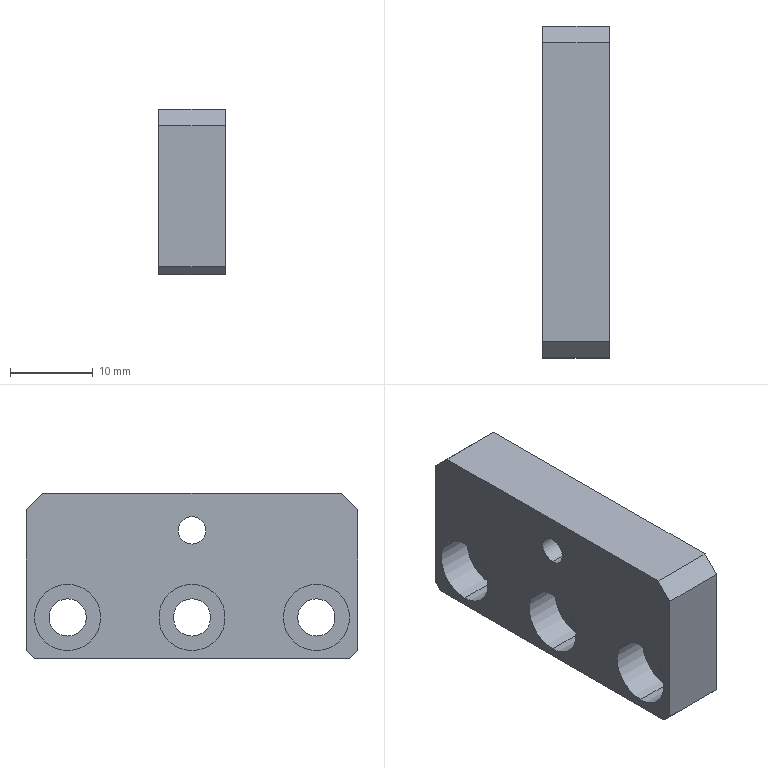Part | STEP file | 11-FG-E04511 | 1 solid | 27 faces | box 8 x 40 x 20 mm | volume 5456 mm3 | cylinder 14 | plane 13 | commonest cylinder face diameters 4.5 x6 8 x6 3.3 x2
STEP:
#1=CARTESIAN_POINT('',(4.,0.,13.85));
#2=VERTEX_POINT('',#1);
#3=CARTESIAN_POINT('',(4.,0.,17.15));
#4=VERTEX_POINT('',#3);
#5=CARTESIAN_POINT('',(4.,0.,15.5));
#6=DIRECTION('',(-1.,0.,0.));
#7=DIRECTION('',(0.,-1.,0.));
#8=AXIS2_PLACEMENT_3D('',#5,#6,#7);
#9=CIRCLE('',#8,1.65);
#10=EDGE_CURVE('',#2,#4,#9,.T.);
#11=ORIENTED_EDGE('',*,*,#10,.F.);
#12=CARTESIAN_POINT('',(-4.,0.,13.85));
#13=VERTEX_POINT('',#12);
#14=CARTESIAN_POINT('',(-4.,0.,13.85));
#15=DIRECTION('',(-1.,0.,0.));
#16=VECTOR('',#15,1000.);
#17=LINE('',#14,#16);
#18=EDGE_CURVE('',#2,#13,#17,.T.);
#19=ORIENTED_EDGE('',*,*,#18,.T.);
#20=CARTESIAN_POINT('',(-4.,0.,17.15));
#21=VERTEX_POINT('',#20);
#22=CARTESIAN_POINT('',(-4.,0.,15.5));
#23=DIRECTION('',(-1.,0.,0.));
#24=DIRECTION('',(0.,0.,1.));
#25=AXIS2_PLACEMENT_3D('',#22,#23,#24);
#26=CIRCLE('',#25,1.65);
#27=EDGE_CURVE('',#13,#21,#26,.T.);
#28=ORIENTED_EDGE('',*,*,#27,.T.);
#29=CARTESIAN_POINT('',(-4.,0.,17.15));
#30=DIRECTION('',(-1.,0.,0.));
#31=VECTOR('',#30,1000.);
#32=LINE('',#29,#31);
#33=EDGE_CURVE('',#4,#21,#32,.T.);
#34=ORIENTED_EDGE('',*,*,#33,.F.);
#35=EDGE_LOOP('',(#11,#19,#28,#34));
#36=FACE_OUTER_BOUND('',#35,.T.);
#37=CARTESIAN_POINT('',(-4.,0.,15.5));
#38=DIRECTION('',(-1.,0.,0.));
#39=DIRECTION('',(0.,0.,1.));
#40=AXIS2_PLACEMENT_3D('',#37,#38,#39);
#41=CYLINDRICAL_SURFACE('',#40,1.65);
#42=ADVANCED_FACE('',(#36),#41,.F.);
#43=CARTESIAN_POINT('',(0.4,15.,1.));
#44=VERTEX_POINT('',#43);
#45=CARTESIAN_POINT('',(0.4,15.,9.));
#46=VERTEX_POINT('',#45);
#47=CARTESIAN_POINT('',(0.4,15.,5.));
#48=DIRECTION('',(-1.,0.,0.));
#49=DIRECTION('',(0.,0.,1.));
#50=AXIS2_PLACEMENT_3D('',#47,#48,#49);
#51=CIRCLE('',#50,4.);
#52=EDGE_CURVE('',#44,#46,#51,.T.);
#53=ORIENTED_EDGE('',*,*,#52,.F.);
#54=CARTESIAN_POINT('',(-4.,15.,1.));
#55=VERTEX_POINT('',#54);
#56=CARTESIAN_POINT('',(-4.,15.,1.));
#57=DIRECTION('',(-1.,0.,0.));
#58=VECTOR('',#57,1000.);
#59=LINE('',#56,#58);
#60=EDGE_CURVE('',#44,#55,#59,.T.);
#61=ORIENTED_EDGE('',*,*,#60,.T.);
#62=CARTESIAN_POINT('',(-4.,15.,9.));
#63=VERTEX_POINT('',#62);
#64=CARTESIAN_POINT('',(-4.,15.,5.));
#65=DIRECTION('',(-1.,0.,0.));
#66=DIRECTION('',(0.,0.,1.));
#67=AXIS2_PLACEMENT_3D('',#64,#65,#66);
#68=CIRCLE('',#67,4.);
#69=EDGE_CURVE('',#55,#63,#68,.T.);
#70=ORIENTED_EDGE('',*,*,#69,.T.);
#71=CARTESIAN_POINT('',(-4.,15.,9.));
#72=DIRECTION('',(-1.,0.,0.));
#73=VECTOR('',#72,1000.);
#74=LINE('',#71,#73);
#75=EDGE_CURVE('',#46,#63,#74,.T.);
#76=ORIENTED_EDGE('',*,*,#75,.F.);
#77=EDGE_LOOP('',(#53,#61,#70,#76));
#78=FACE_OUTER_BOUND('',#77,.T.);
#79=CARTESIAN_POINT('',(-4.,15.,5.));
#80=DIRECTION('',(-1.,0.,0.));
#81=DIRECTION('',(0.,0.,1.));
#82=AXIS2_PLACEMENT_3D('',#79,#80,#81);
#83=CYLINDRICAL_SURFACE('',#82,4.);
#84=ADVANCED_FACE('',(#78),#83,.F.);
#85=CARTESIAN_POINT('',(4.,15.,2.75));
#86=VERTEX_POINT('',#85);
#87=CARTESIAN_POINT('',(4.,15.,7.25));
#88=VERTEX_POINT('',#87);
#89=CARTESIAN_POINT('',(4.,15.,5.));
#90=DIRECTION('',(-1.,0.,0.));
#91=DIRECTION('',(0.,-1.,0.));
#92=AXIS2_PLACEMENT_3D('',#89,#90,#91);
#93=CIRCLE('',#92,2.25);
#94=EDGE_CURVE('',#86,#88,#93,.T.);
#95=ORIENTED_EDGE('',*,*,#94,.F.);
#96=CARTESIAN_POINT('',(0.4,15.,2.75));
#97=VERTEX_POINT('',#96);
#98=CARTESIAN_POINT('',(-4.,15.,2.75));
#99=DIRECTION('',(-1.,0.,0.));
#100=VECTOR('',#99,1000.);
#101=LINE('',#98,#100);
#102=EDGE_CURVE('',#86,#97,#101,.T.);
#103=ORIENTED_EDGE('',*,*,#102,.T.);
#104=CARTESIAN_POINT('',(0.4,15.,7.25));
#105=VERTEX_POINT('',#104);
#106=CARTESIAN_POINT('',(0.4,15.,5.));
#107=DIRECTION('',(-1.,0.,0.));
#108=DIRECTION('',(0.,0.,1.));
#109=AXIS2_PLACEMENT_3D('',#106,#107,#108);
#110=CIRCLE('',#109,2.25);
#111=EDGE_CURVE('',#97,#105,#110,.T.);
#112=ORIENTED_EDGE('',*,*,#111,.T.);
#113=CARTESIAN_POINT('',(-4.,15.,7.25));
#114=DIRECTION('',(-1.,0.,0.));
#115=VECTOR('',#114,1000.);
#116=LINE('',#113,#115);
#117=EDGE_CURVE('',#88,#105,#116,.T.);
#118=ORIENTED_EDGE('',*,*,#117,.F.);
#119=EDGE_LOOP('',(#95,#103,#112,#118));
#120=FACE_OUTER_BOUND('',#119,.T.);
#121=CARTESIAN_POINT('',(-4.,15.,5.));
#122=DIRECTION('',(-1.,0.,0.));
#123=DIRECTION('',(0.,0.,1.));
#124=AXIS2_PLACEMENT_3D('',#121,#122,#123);
#125=CYLINDRICAL_SURFACE('',#124,2.25);
#126=ADVANCED_FACE('',(#120),#125,.F.);
#127=CARTESIAN_POINT('',(0.4,0.,1.));
#128=VERTEX_POINT('',#127);
#129=CARTESIAN_POINT('',(0.4,0.,9.));
#130=VERTEX_POINT('',#129);
#131=CARTESIAN_POINT('',(0.4,0.,5.));
#132=DIRECTION('',(-1.,0.,0.));
#133=DIRECTION('',(0.,0.,1.));
#134=AXIS2_PLACEMENT_3D('',#131,#132,#133);
#135=CIRCLE('',#134,4.);
#136=EDGE_CURVE('',#128,#130,#135,.T.);
#137=ORIENTED_EDGE('',*,*,#136,.F.);
#138=CARTESIAN_POINT('',(-4.,0.,1.));
#139=VERTEX_POINT('',#138);
#140=CARTESIAN_POINT('',(-4.,0.,1.));
#141=DIRECTION('',(-1.,0.,0.));
#142=VECTOR('',#141,1000.);
#143=LINE('',#140,#142);
#144=EDGE_CURVE('',#128,#139,#143,.T.);
#145=ORIENTED_EDGE('',*,*,#144,.T.);
#146=CARTESIAN_POINT('',(-4.,0.,9.));
#147=VERTEX_POINT('',#146);
#148=CARTESIAN_POINT('',(-4.,0.,5.));
#149=DIRECTION('',(-1.,0.,0.));
#150=DIRECTION('',(0.,0.,1.));
#151=AXIS2_PLACEMENT_3D('',#148,#149,#150);
#152=CIRCLE('',#151,4.);
#153=EDGE_CURVE('',#139,#147,#152,.T.);
#154=ORIENTED_EDGE('',*,*,#153,.T.);
#155=CARTESIAN_POINT('',(-4.,0.,9.));
#156=DIRECTION('',(-1.,0.,0.));
#157=VECTOR('',#156,1000.);
#158=LINE('',#155,#157);
#159=EDGE_CURVE('',#130,#147,#158,.T.);
#160=ORIENTED_EDGE('',*,*,#159,.F.);
#161=EDGE_LOOP('',(#137,#145,#154,#160));
#162=FACE_OUTER_BOUND('',#161,.T.);
#163=CARTESIAN_POINT('',(-4.,0.,5.));
#164=DIRECTION('',(-1.,0.,0.));
#165=DIRECTION('',(0.,0.,1.));
#166=AXIS2_PLACEMENT_3D('',#163,#164,#165);
#167=CYLINDRICAL_SURFACE('',#166,4.);
#168=ADVANCED_FACE('',(#162),#167,.F.);
#169=CARTESIAN_POINT('',(4.,0.,2.75));
#170=VERTEX_POINT('',#169);
#171=CARTESIAN_POINT('',(4.,0.,7.25));
#172=VERTEX_POINT('',#171);
#173=CARTESIAN_POINT('',(4.,0.,5.));
#174=DIRECTION('',(-1.,0.,0.));
#175=DIRECTION('',(0.,-1.,0.));
#176=AXIS2_PLACEMENT_3D('',#173,#174,#175);
#177=CIRCLE('',#176,2.25);
#178=EDGE_CURVE('',#170,#172,#177,.T.);
#179=ORIENTED_EDGE('',*,*,#178,.F.);
#180=CARTESIAN_POINT('',(0.4,0.,2.75));
#181=VERTEX_POINT('',#180);
#182=CARTESIAN_POINT('',(-4.,0.,2.75));
#183=DIRECTION('',(-1.,0.,0.));
#184=VECTOR('',#183,1000.);
#185=LINE('',#182,#184);
#186=EDGE_CURVE('',#170,#181,#185,.T.);
#187=ORIENTED_EDGE('',*,*,#186,.T.);
#188=CARTESIAN_POINT('',(0.4,0.,7.25));
#189=VERTEX_POINT('',#188);
#190=CARTESIAN_POINT('',(0.4,0.,5.));
#191=DIRECTION('',(-1.,0.,0.));
#192=DIRECTION('',(0.,0.,1.));
#193=AXIS2_PLACEMENT_3D('',#190,#191,#192);
#194=CIRCLE('',#193,2.25);
#195=EDGE_CURVE('',#181,#189,#194,.T.);
#196=ORIENTED_EDGE('',*,*,#195,.T.);
#197=CARTESIAN_POINT('',(-4.,0.,7.25));
#198=DIRECTION('',(-1.,0.,0.));
#199=VECTOR('',#198,1000.);
#200=LINE('',#197,#199);
#201=EDGE_CURVE('',#172,#189,#200,.T.);
#202=ORIENTED_EDGE('',*,*,#201,.F.);
#203=EDGE_LOOP('',(#179,#187,#196,#202));
#204=FACE_OUTER_BOUND('',#203,.T.);
#205=CARTESIAN_POINT('',(-4.,0.,5.));
#206=DIRECTION('',(-1.,0.,0.));
#207=DIRECTION('',(0.,0.,1.));
#208=AXIS2_PLACEMENT_3D('',#205,#206,#207);
#209=CYLINDRICAL_SURFACE('',#208,2.25);
#210=ADVANCED_FACE('',(#204),#209,.F.);
#211=CARTESIAN_POINT('',(0.4,-15.,1.));
#212=VERTEX_POINT('',#211);
#213=CARTESIAN_POINT('',(0.4,-15.,9.));
#214=VERTEX_POINT('',#213);
#215=CARTESIAN_POINT('',(0.4,-15.,5.));
#216=DIRECTION('',(-1.,0.,0.));
#217=DIRECTION('',(0.,0.,1.));
#218=AXIS2_PLACEMENT_3D('',#215,#216,#217);
#219=CIRCLE('',#218,4.);
#220=EDGE_CURVE('',#212,#214,#219,.T.);
#221=ORIENTED_EDGE('',*,*,#220,.F.);
#222=CARTESIAN_POINT('',(-4.,-15.,1.));
#223=VERTEX_POINT('',#222);
#224=CARTESIAN_POINT('',(-4.,-15.,1.));
#225=DIRECTION('',(-1.,0.,0.));
#226=VECTOR('',#225,1000.);
#227=LINE('',#224,#226);
#228=EDGE_CURVE('',#212,#223,#227,.T.);
#229=ORIENTED_EDGE('',*,*,#228,.T.);
#230=CARTESIAN_POINT('',(-4.,-15.,9.));
#231=VERTEX_POINT('',#230);
#232=CARTESIAN_POINT('',(-4.,-15.,5.));
#233=DIRECTION('',(-1.,0.,0.));
#234=DIRECTION('',(0.,0.,1.));
#235=AXIS2_PLACEMENT_3D('',#232,#233,#234);
#236=CIRCLE('',#235,4.);
#237=EDGE_CURVE('',#223,#231,#236,.T.);
#238=ORIENTED_EDGE('',*,*,#237,.T.);
#239=CARTESIAN_POINT('',(-4.,-15.,9.));
#240=DIRECTION('',(-1.,0.,0.));
#241=VECTOR('',#240,1000.);
#242=LINE('',#239,#241);
#243=EDGE_CURVE('',#214,#231,#242,.T.);
#244=ORIENTED_EDGE('',*,*,#243,.F.);
#245=EDGE_LOOP('',(#221,#229,#238,#244));
#246=FACE_OUTER_BOUND('',#245,.T.);
#247=CARTESIAN_POINT('',(-4.,-15.,5.));
#248=DIRECTION('',(-1.,0.,0.));
#249=DIRECTION('',(0.,0.,1.));
#250=AXIS2_PLACEMENT_3D('',#247,#248,#249);
#251=CYLINDRICAL_SURFACE('',#250,4.);
#252=ADVANCED_FACE('',(#246),#251,.F.);
#253=CARTESIAN_POINT('',(4.,-15.,2.75));
#254=VERTEX_POINT('',#253);
#255=CARTESIAN_POINT('',(4.,-15.,7.25));
#256=VERTEX_POINT('',#255);
#257=CARTESIAN_POINT('',(4.,-15.,5.));
#258=DIRECTION('',(-1.,0.,0.));
#259=DIRECTION('',(0.,-1.,0.));
#260=AXIS2_PLACEMENT_3D('',#257,#258,#259);
#261=CIRCLE('',#260,2.25);
#262=EDGE_CURVE('',#254,#256,#261,.T.);
#263=ORIENTED_EDGE('',*,*,#262,.F.);
#264=CARTESIAN_POINT('',(0.4,-15.,2.75));
#265=VERTEX_POINT('',#264);
#266=CARTESIAN_POINT('',(-4.,-15.,2.75));
#267=DIRECTION('',(-1.,0.,0.));
#268=VECTOR('',#267,1000.);
#269=LINE('',#266,#268);
#270=EDGE_CURVE('',#254,#265,#269,.T.);
#271=ORIENTED_EDGE('',*,*,#270,.T.);
#272=CARTESIAN_POINT('',(0.4,-15.,7.25));
#273=VERTEX_POINT('',#272);
#274=CARTESIAN_POINT('',(0.4,-15.,5.));
#275=DIRECTION('',(-1.,0.,0.));
#276=DIRECTION('',(0.,0.,1.));
#277=AXIS2_PLACEMENT_3D('',#274,#275,#276);
#278=CIRCLE('',#277,2.25);
#279=EDGE_CURVE('',#265,#273,#278,.T.);
#280=ORIENTED_EDGE('',*,*,#279,.T.);
#281=CARTESIAN_POINT('',(-4.,-15.,7.25));
#282=DIRECTION('',(-1.,0.,0.));
#283=VECTOR('',#282,1000.);
#284=LINE('',#281,#283);
#285=EDGE_CURVE('',#256,#273,#284,.T.);
#286=ORIENTED_EDGE('',*,*,#285,.F.);
#287=EDGE_LOOP('',(#263,#271,#280,#286));
#288=FACE_OUTER_BOUND('',#287,.T.);
#289=CARTESIAN_POINT('',(-4.,-15.,5.));
#290=DIRECTION('',(-1.,0.,0.));
#291=DIRECTION('',(0.,0.,1.));
#292=AXIS2_PLACEMENT_3D('',#289,#290,#291);
#293=CYLINDRICAL_SURFACE('',#292,2.25);
#294=ADVANCED_FACE('',(#288),#293,.F.);
#295=CARTESIAN_POINT('',(4.,0.,15.5));
#296=DIRECTION('',(-1.,0.,0.));
#297=DIRECTION('',(0.,-1.,0.));
#298=AXIS2_PLACEMENT_3D('',#295,#296,#297);
#299=CIRCLE('',#298,1.65);
#300=EDGE_CURVE('',#4,#2,#299,.T.);
#301=ORIENTED_EDGE('',*,*,#300,.T.);
#302=ORIENTED_EDGE('',*,*,#10,.T.);
#303=EDGE_LOOP('',(#301,#302));
#304=FACE_BOUND('',#303,.T.);
#305=CARTESIAN_POINT('',(4.,15.,5.));
#306=DIRECTION('',(-1.,0.,0.));
#307=DIRECTION('',(0.,-1.,0.));
#308=AXIS2_PLACEMENT_3D('',#305,#306,#307);
#309=CIRCLE('',#308,2.25);
#310=EDGE_CURVE('',#88,#86,#309,.T.);
#311=ORIENTED_EDGE('',*,*,#310,.T.);
#312=ORIENTED_EDGE('',*,*,#94,.T.);
#313=EDGE_LOOP('',(#311,#312));
#314=FACE_BOUND('',#313,.T.);
#315=CARTESIAN_POINT('',(4.,0.,5.));
#316=DIRECTION('',(-1.,0.,0.));
#317=DIRECTION('',(0.,-1.,0.));
#318=AXIS2_PLACEMENT_3D('',#315,#316,#317);
#319=CIRCLE('',#318,2.25);
#320=EDGE_CURVE('',#172,#170,#319,.T.);
#321=ORIENTED_EDGE('',*,*,#320,.T.);
#322=ORIENTED_EDGE('',*,*,#178,.T.);
#323=EDGE_LOOP('',(#321,#322));
#324=FACE_BOUND('',#323,.T.);
#325=CARTESIAN_POINT('',(4.,-15.,5.));
#326=DIRECTION('',(-1.,0.,0.));
#327=DIRECTION('',(0.,-1.,0.));
#328=AXIS2_PLACEMENT_3D('',#325,#326,#327);
#329=CIRCLE('',#328,2.25);
#330=EDGE_CURVE('',#256,#254,#329,.T.);
#331=ORIENTED_EDGE('',*,*,#330,.T.);
#332=ORIENTED_EDGE('',*,*,#262,.T.);
#333=EDGE_LOOP('',(#331,#332));
#334=FACE_BOUND('',#333,.T.);
#335=CARTESIAN_POINT('',(4.,-20.,18.));
#336=VERTEX_POINT('',#335);
#337=CARTESIAN_POINT('',(4.,-20.,1.));
#338=VERTEX_POINT('',#337);
#339=CARTESIAN_POINT('',(4.,-20.,20.));
#340=DIRECTION('',(0.,0.,-1.));
#341=VECTOR('',#340,1000.);
#342=LINE('',#339,#341);
#343=EDGE_CURVE('',#336,#338,#342,.T.);
#344=ORIENTED_EDGE('',*,*,#343,.T.);
#345=CARTESIAN_POINT('',(4.,-19.,0.));
#346=VERTEX_POINT('',#345);
#347=CARTESIAN_POINT('',(4.,-20.,1.));
#348=DIRECTION('',(0.,0.7071,-0.7071));
#349=VECTOR('',#348,1000.);
#350=LINE('',#347,#349);
#351=EDGE_CURVE('',#338,#346,#350,.T.);
#352=ORIENTED_EDGE('',*,*,#351,.T.);
#353=CARTESIAN_POINT('',(4.,19.,0.));
#354=VERTEX_POINT('',#353);
#355=CARTESIAN_POINT('',(4.,20.,0.));
#356=DIRECTION('',(0.,1.,0.));
#357=VECTOR('',#356,1000.);
#358=LINE('',#355,#357);
#359=EDGE_CURVE('',#346,#354,#358,.T.);
#360=ORIENTED_EDGE('',*,*,#359,.T.);
#361=CARTESIAN_POINT('',(4.,20.,1.));
#362=VERTEX_POINT('',#361);
#363=CARTESIAN_POINT('',(4.,20.,1.));
#364=DIRECTION('',(0.,0.7071,0.7071));
#365=VECTOR('',#364,1000.);
#366=LINE('',#363,#365);
#367=EDGE_CURVE('',#354,#362,#366,.T.);
#368=ORIENTED_EDGE('',*,*,#367,.T.);
#369=CARTESIAN_POINT('',(4.,20.,18.));
#370=VERTEX_POINT('',#369);
#371=CARTESIAN_POINT('',(4.,20.,20.));
#372=DIRECTION('',(0.,0.,-1.));
#373=VECTOR('',#372,1000.);
#374=LINE('',#371,#373);
#375=EDGE_CURVE('',#370,#362,#374,.T.);
#376=ORIENTED_EDGE('',*,*,#375,.F.);
#377=CARTESIAN_POINT('',(4.,18.,20.));
#378=VERTEX_POINT('',#377);
#379=CARTESIAN_POINT('',(4.,18.,20.));
#380=DIRECTION('',(0.,-0.7071,0.7071));
#381=VECTOR('',#380,1000.);
#382=LINE('',#379,#381);
#383=EDGE_CURVE('',#370,#378,#382,.T.);
#384=ORIENTED_EDGE('',*,*,#383,.T.);
#385=CARTESIAN_POINT('',(4.,-18.,20.));
#386=VERTEX_POINT('',#385);
#387=CARTESIAN_POINT('',(4.,20.,20.));
#388=DIRECTION('',(0.,1.,0.));
#389=VECTOR('',#388,1000.);
#390=LINE('',#387,#389);
#391=EDGE_CURVE('',#386,#378,#390,.T.);
#392=ORIENTED_EDGE('',*,*,#391,.F.);
#393=CARTESIAN_POINT('',(4.,-18.,20.));
#394=DIRECTION('',(0.,-0.7071,-0.7071));
#395=VECTOR('',#394,1000.);
#396=LINE('',#393,#395);
#397=EDGE_CURVE('',#386,#336,#396,.T.);
#398=ORIENTED_EDGE('',*,*,#397,.T.);
#399=EDGE_LOOP('',(#344,#352,#360,#368,#376,#384,#392,#398));
#400=FACE_OUTER_BOUND('',#399,.T.);
#401=CARTESIAN_POINT('',(4.,20.,20.));
#402=DIRECTION('',(-1.,0.,0.));
#403=DIRECTION('',(0.,-1.,0.));
#404=AXIS2_PLACEMENT_3D('',#401,#402,#403);
#405=PLANE('',#404);
#406=ADVANCED_FACE('',(#304,#314,#324,#334,#400),#405,.F.);
#407=ORIENTED_EDGE('',*,*,#375,.T.);
#408=CARTESIAN_POINT('',(-4.,20.,1.));
#409=VERTEX_POINT('',#408);
#410=CARTESIAN_POINT('',(-4.,20.,1.));
#411=DIRECTION('',(-1.,0.,0.));
#412=VECTOR('',#411,1000.);
#413=LINE('',#410,#412);
#414=EDGE_CURVE('',#362,#409,#413,.T.);
#415=ORIENTED_EDGE('',*,*,#414,.T.);
#416=CARTESIAN_POINT('',(-4.,20.,18.));
#417=VERTEX_POINT('',#416);
#418=CARTESIAN_POINT('',(-4.,20.,20.));
#419=DIRECTION('',(0.,0.,-1.));
#420=VECTOR('',#419,1000.);
#421=LINE('',#418,#420);
#422=EDGE_CURVE('',#417,#409,#421,.T.);
#423=ORIENTED_EDGE('',*,*,#422,.F.);
#424=CARTESIAN_POINT('',(4.,20.,18.));
#425=DIRECTION('',(1.,0.,0.));
#426=VECTOR('',#425,1000.);
#427=LINE('',#424,#426);
#428=EDGE_CURVE('',#417,#370,#427,.T.);
#429=ORIENTED_EDGE('',*,*,#428,.T.);
#430=EDGE_LOOP('',(#407,#415,#423,#429));
#431=FACE_OUTER_BOUND('',#430,.T.);
#432=CARTESIAN_POINT('',(-4.,20.,20.));
#433=DIRECTION('',(0.,-1.,0.));
#434=DIRECTION('',(0.,0.,-1.));
#435=AXIS2_PLACEMENT_3D('',#432,#433,#434);
#436=PLANE('',#435);
#437=ADVANCED_FACE('',(#431),#436,.F.);
#438=CARTESIAN_POINT('',(-4.,0.,15.5));
#439=DIRECTION('',(-1.,0.,0.));
#440=DIRECTION('',(0.,0.,1.));
#441=AXIS2_PLACEMENT_3D('',#438,#439,#440);
#442=CIRCLE('',#441,1.65);
#443=EDGE_CURVE('',#21,#13,#442,.T.);
#444=ORIENTED_EDGE('',*,*,#443,.F.);
#445=ORIENTED_EDGE('',*,*,#27,.F.);
#446=EDGE_LOOP('',(#444,#445));
#447=FACE_BOUND('',#446,.T.);
#448=CARTESIAN_POINT('',(-4.,15.,5.));
#449=DIRECTION('',(-1.,0.,0.));
#450=DIRECTION('',(0.,0.,1.));
#451=AXIS2_PLACEMENT_3D('',#448,#449,#450);
#452=CIRCLE('',#451,4.);
#453=EDGE_CURVE('',#63,#55,#452,.T.);
#454=ORIENTED_EDGE('',*,*,#453,.F.);
#455=ORIENTED_EDGE('',*,*,#69,.F.);
#456=EDGE_LOOP('',(#454,#455));
#457=FACE_BOUND('',#456,.T.);
#458=CARTESIAN_POINT('',(-4.,0.,5.));
#459=DIRECTION('',(-1.,0.,0.));
#460=DIRECTION('',(0.,0.,1.));
#461=AXIS2_PLACEMENT_3D('',#458,#459,#460);
#462=CIRCLE('',#461,4.);
#463=EDGE_CURVE('',#147,#139,#462,.T.);
#464=ORIENTED_EDGE('',*,*,#463,.F.);
#465=ORIENTED_EDGE('',*,*,#153,.F.);
#466=EDGE_LOOP('',(#464,#465));
#467=FACE_BOUND('',#466,.T.);
#468=CARTESIAN_POINT('',(-4.,-15.,5.));
#469=DIRECTION('',(-1.,0.,0.));
#470=DIRECTION('',(0.,0.,1.));
#471=AXIS2_PLACEMENT_3D('',#468,#469,#470);
#472=CIRCLE('',#471,4.);
#473=EDGE_CURVE('',#231,#223,#472,.T.);
#474=ORIENTED_EDGE('',*,*,#473,.F.);
#475=ORIENTED_EDGE('',*,*,#237,.F.);
#476=EDGE_LOOP('',(#474,#475));
#477=FACE_BOUND('',#476,.T.);
#478=CARTESIAN_POINT('',(-4.,19.,0.));
#479=VERTEX_POINT('',#478);
#480=CARTESIAN_POINT('',(-4.,-19.,0.));
#481=VERTEX_POINT('',#480);
#482=CARTESIAN_POINT('',(-4.,20.,0.));
#483=DIRECTION('',(0.,-1.,0.));
#484=VECTOR('',#483,1000.);
#485=LINE('',#482,#484);
#486=EDGE_CURVE('',#479,#481,#485,.T.);
#487=ORIENTED_EDGE('',*,*,#486,.T.);
#488=CARTESIAN_POINT('',(-4.,-20.,1.));
#489=VERTEX_POINT('',#488);
#490=CARTESIAN_POINT('',(-4.,-20.,1.));
#491=DIRECTION('',(0.,-0.7071,0.7071));
#492=VECTOR('',#491,1000.);
#493=LINE('',#490,#492);
#494=EDGE_CURVE('',#481,#489,#493,.T.);
#495=ORIENTED_EDGE('',*,*,#494,.T.);
#496=CARTESIAN_POINT('',(-4.,-20.,18.));
#497=VERTEX_POINT('',#496);
#498=CARTESIAN_POINT('',(-4.,-20.,20.));
#499=DIRECTION('',(0.,0.,-1.));
#500=VECTOR('',#499,1000.);
#501=LINE('',#498,#500);
#502=EDGE_CURVE('',#497,#489,#501,.T.);
#503=ORIENTED_EDGE('',*,*,#502,.F.);
#504=CARTESIAN_POINT('',(-4.,-18.,20.));
#505=VERTEX_POINT('',#504);
#506=CARTESIAN_POINT('',(-4.,-18.,20.));
#507=DIRECTION('',(0.,0.7071,0.7071));
#508=VECTOR('',#507,1000.);
#509=LINE('',#506,#508);
#510=EDGE_CURVE('',#497,#505,#509,.T.);
#511=ORIENTED_EDGE('',*,*,#510,.T.);
#512=CARTESIAN_POINT('',(-4.,18.,20.));
#513=VERTEX_POINT('',#512);
#514=CARTESIAN_POINT('',(-4.,20.,20.));
#515=DIRECTION('',(0.,-1.,0.));
#516=VECTOR('',#515,1000.);
#517=LINE('',#514,#516);
#518=EDGE_CURVE('',#513,#505,#517,.T.);
#519=ORIENTED_EDGE('',*,*,#518,.F.);
#520=CARTESIAN_POINT('',(-4.,18.,20.));
#521=DIRECTION('',(0.,0.7071,-0.7071));
#522=VECTOR('',#521,1000.);
#523=LINE('',#520,#522);
#524=EDGE_CURVE('',#513,#417,#523,.T.);
#525=ORIENTED_EDGE('',*,*,#524,.T.);
#526=ORIENTED_EDGE('',*,*,#422,.T.);
#527=CARTESIAN_POINT('',(-4.,20.,1.));
#528=DIRECTION('',(0.,-0.7071,-0.7071));
#529=VECTOR('',#528,1000.);
#530=LINE('',#527,#529);
#531=EDGE_CURVE('',#409,#479,#530,.T.);
#532=ORIENTED_EDGE('',*,*,#531,.T.);
#533=EDGE_LOOP('',(#487,#495,#503,#511,#519,#525,#526,#532));
#534=FACE_OUTER_BOUND('',#533,.T.);
#535=CARTESIAN_POINT('',(-4.,20.,20.));
#536=DIRECTION('',(1.,0.,0.));
#537=DIRECTION('',(0.,1.,0.));
#538=AXIS2_PLACEMENT_3D('',#535,#536,#537);
#539=PLANE('',#538);
#540=ADVANCED_FACE('',(#447,#457,#467,#477,#534),#539,.F.);
#541=ORIENTED_EDGE('',*,*,#502,.T.);
#542=CARTESIAN_POINT('',(-4.,-20.,1.));
#543=DIRECTION('',(1.,0.,0.));
#544=VECTOR('',#543,1000.);
#545=LINE('',#542,#544);
#546=EDGE_CURVE('',#489,#338,#545,.T.);
#547=ORIENTED_EDGE('',*,*,#546,.T.);
#548=ORIENTED_EDGE('',*,*,#343,.F.);
#549=CARTESIAN_POINT('',(-4.,-20.,18.));
#550=DIRECTION('',(-1.,0.,0.));
#551=VECTOR('',#550,1000.);
#552=LINE('',#549,#551);
#553=EDGE_CURVE('',#336,#497,#552,.T.);
#554=ORIENTED_EDGE('',*,*,#553,.T.);
#555=EDGE_LOOP('',(#541,#547,#548,#554));
#556=FACE_OUTER_BOUND('',#555,.T.);
#557=CARTESIAN_POINT('',(-4.,-20.,20.));
#558=DIRECTION('',(0.,1.,0.));
#559=DIRECTION('',(0.,0.,1.));
#560=AXIS2_PLACEMENT_3D('',#557,#558,#559);
#561=PLANE('',#560);
#562=ADVANCED_FACE('',(#556),#561,.F.);
#563=ORIENTED_EDGE('',*,*,#518,.T.);
#564=CARTESIAN_POINT('',(4.,-18.,20.));
#565=DIRECTION('',(1.,0.,0.));
#566=VECTOR('',#565,1000.);
#567=LINE('',#564,#566);
#568=EDGE_CURVE('',#505,#386,#567,.T.);
#569=ORIENTED_EDGE('',*,*,#568,.T.);
#570=ORIENTED_EDGE('',*,*,#391,.T.);
#571=CARTESIAN_POINT('',(-4.,18.,20.));
#572=DIRECTION('',(-1.,0.,0.));
#573=VECTOR('',#572,1000.);
#574=LINE('',#571,#573);
#575=EDGE_CURVE('',#378,#513,#574,.T.);
#576=ORIENTED_EDGE('',*,*,#575,.T.);
#577=EDGE_LOOP('',(#563,#569,#570,#576));
#578=FACE_OUTER_BOUND('',#577,.T.);
#579=CARTESIAN_POINT('',(0.,0.,20.));
#580=DIRECTION('',(0.,0.,1.));
#581=DIRECTION('',(1.,0.,0.));
#582=AXIS2_PLACEMENT_3D('',#579,#580,#581);
#583=PLANE('',#582);
#584=ADVANCED_FACE('',(#578),#583,.T.);
#585=ORIENTED_EDGE('',*,*,#359,.F.);
#586=CARTESIAN_POINT('',(0.,-19.,0.));
#587=DIRECTION('',(-1.,0.,0.));
#588=VECTOR('',#587,1000.);
#589=LINE('',#586,#588);
#590=EDGE_CURVE('',#346,#481,#589,.T.);
#591=ORIENTED_EDGE('',*,*,#590,.T.);
#592=ORIENTED_EDGE('',*,*,#486,.F.);
#593=CARTESIAN_POINT('',(0.,19.,0.));
#594=DIRECTION('',(1.,0.,0.));
#595=VECTOR('',#594,1000.);
#596=LINE('',#593,#595);
#597=EDGE_CURVE('',#479,#354,#596,.T.);
#598=ORIENTED_EDGE('',*,*,#597,.T.);
#599=EDGE_LOOP('',(#585,#591,#592,#598));
#600=FACE_OUTER_BOUND('',#599,.T.);
#601=CARTESIAN_POINT('',(0.,0.,0.));
#602=DIRECTION('',(0.,0.,1.));
#603=DIRECTION('',(1.,0.,0.));
#604=AXIS2_PLACEMENT_3D('',#601,#602,#603);
#605=PLANE('',#604);
#606=ADVANCED_FACE('',(#600),#605,.F.);
#607=ORIENTED_EDGE('',*,*,#270,.F.);
#608=ORIENTED_EDGE('',*,*,#330,.F.);
#609=ORIENTED_EDGE('',*,*,#285,.T.);
#610=CARTESIAN_POINT('',(0.4,-15.,5.));
#611=DIRECTION('',(-1.,0.,0.));
#612=DIRECTION('',(0.,0.,1.));
#613=AXIS2_PLACEMENT_3D('',#610,#611,#612);
#614=CIRCLE('',#613,2.25);
#615=EDGE_CURVE('',#273,#265,#614,.T.);
#616=ORIENTED_EDGE('',*,*,#615,.T.);
#617=EDGE_LOOP('',(#607,#608,#609,#616));
#618=FACE_OUTER_BOUND('',#617,.T.);
#619=CARTESIAN_POINT('',(-4.,-15.,5.));
#620=DIRECTION('',(-1.,0.,0.));
#621=DIRECTION('',(0.,0.,1.));
#622=AXIS2_PLACEMENT_3D('',#619,#620,#621);
#623=CYLINDRICAL_SURFACE('',#622,2.25);
#624=ADVANCED_FACE('',(#618),#623,.F.);
#625=ORIENTED_EDGE('',*,*,#615,.F.);
#626=ORIENTED_EDGE('',*,*,#279,.F.);
#627=EDGE_LOOP('',(#625,#626));
#628=FACE_BOUND('',#627,.T.);
#629=CARTESIAN_POINT('',(0.4,-15.,5.));
#630=DIRECTION('',(-1.,0.,0.));
#631=DIRECTION('',(0.,0.,1.));
#632=AXIS2_PLACEMENT_3D('',#629,#630,#631);
#633=CIRCLE('',#632,4.);
#634=EDGE_CURVE('',#214,#212,#633,.T.);
#635=ORIENTED_EDGE('',*,*,#634,.T.);
#636=ORIENTED_EDGE('',*,*,#220,.T.);
#637=EDGE_LOOP('',(#635,#636));
#638=FACE_OUTER_BOUND('',#637,.T.);
#639=CARTESIAN_POINT('',(0.4,-12.75,5.));
#640=DIRECTION('',(1.,0.,0.));
#641=DIRECTION('',(0.,0.,-1.));
#642=AXIS2_PLACEMENT_3D('',#639,#640,#641);
#643=PLANE('',#642);
#644=ADVANCED_FACE('',(#628,#638),#643,.F.);
#645=ORIENTED_EDGE('',*,*,#228,.F.);
#646=ORIENTED_EDGE('',*,*,#634,.F.);
#647=ORIENTED_EDGE('',*,*,#243,.T.);
#648=ORIENTED_EDGE('',*,*,#473,.T.);
#649=EDGE_LOOP('',(#645,#646,#647,#648));
#650=FACE_OUTER_BOUND('',#649,.T.);
#651=CARTESIAN_POINT('',(-4.,-15.,5.));
#652=DIRECTION('',(-1.,0.,0.));
#653=DIRECTION('',(0.,0.,1.));
#654=AXIS2_PLACEMENT_3D('',#651,#652,#653);
#655=CYLINDRICAL_SURFACE('',#654,4.);
#656=ADVANCED_FACE('',(#650),#655,.F.);
#657=ORIENTED_EDGE('',*,*,#186,.F.);
#658=ORIENTED_EDGE('',*,*,#320,.F.);
#659=ORIENTED_EDGE('',*,*,#201,.T.);
#660=CARTESIAN_POINT('',(0.4,0.,5.));
#661=DIRECTION('',(-1.,0.,0.));
#662=DIRECTION('',(0.,0.,1.));
#663=AXIS2_PLACEMENT_3D('',#660,#661,#662);
#664=CIRCLE('',#663,2.25);
#665=EDGE_CURVE('',#189,#181,#664,.T.);
#666=ORIENTED_EDGE('',*,*,#665,.T.);
#667=EDGE_LOOP('',(#657,#658,#659,#666));
#668=FACE_OUTER_BOUND('',#667,.T.);
#669=CARTESIAN_POINT('',(-4.,0.,5.));
#670=DIRECTION('',(-1.,0.,0.));
#671=DIRECTION('',(0.,0.,1.));
#672=AXIS2_PLACEMENT_3D('',#669,#670,#671);
#673=CYLINDRICAL_SURFACE('',#672,2.25);
#674=ADVANCED_FACE('',(#668),#673,.F.);
#675=ORIENTED_EDGE('',*,*,#665,.F.);
#676=ORIENTED_EDGE('',*,*,#195,.F.);
#677=EDGE_LOOP('',(#675,#676));
#678=FACE_BOUND('',#677,.T.);
#679=CARTESIAN_POINT('',(0.4,0.,5.));
#680=DIRECTION('',(-1.,0.,0.));
#681=DIRECTION('',(0.,0.,1.));
#682=AXIS2_PLACEMENT_3D('',#679,#680,#681);
#683=CIRCLE('',#682,4.);
#684=EDGE_CURVE('',#130,#128,#683,.T.);
#685=ORIENTED_EDGE('',*,*,#684,.T.);
#686=ORIENTED_EDGE('',*,*,#136,.T.);
#687=EDGE_LOOP('',(#685,#686));
#688=FACE_OUTER_BOUND('',#687,.T.);
#689=CARTESIAN_POINT('',(0.4,2.25,5.));
#690=DIRECTION('',(1.,0.,0.));
#691=DIRECTION('',(0.,0.,-1.));
#692=AXIS2_PLACEMENT_3D('',#689,#690,#691);
#693=PLANE('',#692);
#694=ADVANCED_FACE('',(#678,#688),#693,.F.);
#695=ORIENTED_EDGE('',*,*,#144,.F.);
#696=ORIENTED_EDGE('',*,*,#684,.F.);
#697=ORIENTED_EDGE('',*,*,#159,.T.);
#698=ORIENTED_EDGE('',*,*,#463,.T.);
#699=EDGE_LOOP('',(#695,#696,#697,#698));
#700=FACE_OUTER_BOUND('',#699,.T.);
#701=CARTESIAN_POINT('',(-4.,0.,5.));
#702=DIRECTION('',(-1.,0.,0.));
#703=DIRECTION('',(0.,0.,1.));
#704=AXIS2_PLACEMENT_3D('',#701,#702,#703);
#705=CYLINDRICAL_SURFACE('',#704,4.);
#706=ADVANCED_FACE('',(#700),#705,.F.);
#707=ORIENTED_EDGE('',*,*,#102,.F.);
#708=ORIENTED_EDGE('',*,*,#310,.F.);
#709=ORIENTED_EDGE('',*,*,#117,.T.);
#710=CARTESIAN_POINT('',(0.4,15.,5.));
#711=DIRECTION('',(-1.,0.,0.));
#712=DIRECTION('',(0.,0.,1.));
#713=AXIS2_PLACEMENT_3D('',#710,#711,#712);
#714=CIRCLE('',#713,2.25);
#715=EDGE_CURVE('',#105,#97,#714,.T.);
#716=ORIENTED_EDGE('',*,*,#715,.T.);
#717=EDGE_LOOP('',(#707,#708,#709,#716));
#718=FACE_OUTER_BOUND('',#717,.T.);
#719=CARTESIAN_POINT('',(-4.,15.,5.));
#720=DIRECTION('',(-1.,0.,0.));
#721=DIRECTION('',(0.,0.,1.));
#722=AXIS2_PLACEMENT_3D('',#719,#720,#721);
#723=CYLINDRICAL_SURFACE('',#722,2.25);
#724=ADVANCED_FACE('',(#718),#723,.F.);
#725=ORIENTED_EDGE('',*,*,#715,.F.);
#726=ORIENTED_EDGE('',*,*,#111,.F.);
#727=EDGE_LOOP('',(#725,#726));
#728=FACE_BOUND('',#727,.T.);
#729=CARTESIAN_POINT('',(0.4,15.,5.));
#730=DIRECTION('',(-1.,0.,0.));
#731=DIRECTION('',(0.,0.,1.));
#732=AXIS2_PLACEMENT_3D('',#729,#730,#731);
#733=CIRCLE('',#732,4.);
#734=EDGE_CURVE('',#46,#44,#733,.T.);
#735=ORIENTED_EDGE('',*,*,#734,.T.);
#736=ORIENTED_EDGE('',*,*,#52,.T.);
#737=EDGE_LOOP('',(#735,#736));
#738=FACE_OUTER_BOUND('',#737,.T.);
#739=CARTESIAN_POINT('',(0.4,17.25,5.));
#740=DIRECTION('',(1.,0.,0.));
#741=DIRECTION('',(0.,0.,-1.));
#742=AXIS2_PLACEMENT_3D('',#739,#740,#741);
#743=PLANE('',#742);
#744=ADVANCED_FACE('',(#728,#738),#743,.F.);
#745=ORIENTED_EDGE('',*,*,#60,.F.);
#746=ORIENTED_EDGE('',*,*,#734,.F.);
#747=ORIENTED_EDGE('',*,*,#75,.T.);
#748=ORIENTED_EDGE('',*,*,#453,.T.);
#749=EDGE_LOOP('',(#745,#746,#747,#748));
#750=FACE_OUTER_BOUND('',#749,.T.);
#751=CARTESIAN_POINT('',(-4.,15.,5.));
#752=DIRECTION('',(-1.,0.,0.));
#753=DIRECTION('',(0.,0.,1.));
#754=AXIS2_PLACEMENT_3D('',#751,#752,#753);
#755=CYLINDRICAL_SURFACE('',#754,4.);
#756=ADVANCED_FACE('',(#750),#755,.F.);
#757=ORIENTED_EDGE('',*,*,#18,.F.);
#758=ORIENTED_EDGE('',*,*,#300,.F.);
#759=ORIENTED_EDGE('',*,*,#33,.T.);
#760=ORIENTED_EDGE('',*,*,#443,.T.);
#761=EDGE_LOOP('',(#757,#758,#759,#760));
#762=FACE_OUTER_BOUND('',#761,.T.);
#763=CARTESIAN_POINT('',(-4.,0.,15.5));
#764=DIRECTION('',(-1.,0.,0.));
#765=DIRECTION('',(0.,0.,1.));
#766=AXIS2_PLACEMENT_3D('',#763,#764,#765);
#767=CYLINDRICAL_SURFACE('',#766,1.65);
#768=ADVANCED_FACE('',(#762),#767,.F.);
#769=ORIENTED_EDGE('',*,*,#510,.F.);
#770=ORIENTED_EDGE('',*,*,#553,.F.);
#771=ORIENTED_EDGE('',*,*,#397,.F.);
#772=ORIENTED_EDGE('',*,*,#568,.F.);
#773=EDGE_LOOP('',(#769,#770,#771,#772));
#774=FACE_OUTER_BOUND('',#773,.T.);
#775=CARTESIAN_POINT('',(0.,-18.,20.));
#776=DIRECTION('',(0.,-0.7071,0.7071));
#777=DIRECTION('',(-1.,0.,0.));
#778=AXIS2_PLACEMENT_3D('',#775,#776,#777);
#779=PLANE('',#778);
#780=ADVANCED_FACE('',(#774),#779,.T.);
#781=ORIENTED_EDGE('',*,*,#383,.F.);
#782=ORIENTED_EDGE('',*,*,#428,.F.);
#783=ORIENTED_EDGE('',*,*,#524,.F.);
#784=ORIENTED_EDGE('',*,*,#575,.F.);
#785=EDGE_LOOP('',(#781,#782,#783,#784));
#786=FACE_OUTER_BOUND('',#785,.T.);
#787=CARTESIAN_POINT('',(0.,18.,20.));
#788=DIRECTION('',(0.,0.7071,0.7071));
#789=DIRECTION('',(1.,0.,0.));
#790=AXIS2_PLACEMENT_3D('',#787,#788,#789);
#791=PLANE('',#790);
#792=ADVANCED_FACE('',(#786),#791,.T.);
#793=ORIENTED_EDGE('',*,*,#494,.F.);
#794=ORIENTED_EDGE('',*,*,#590,.F.);
#795=ORIENTED_EDGE('',*,*,#351,.F.);
#796=ORIENTED_EDGE('',*,*,#546,.F.);
#797=EDGE_LOOP('',(#793,#794,#795,#796));
#798=FACE_OUTER_BOUND('',#797,.T.);
#799=CARTESIAN_POINT('',(-4.,-20.,1.));
#800=DIRECTION('',(0.,0.7071,0.7071));
#801=DIRECTION('',(1.,0.,0.));
#802=AXIS2_PLACEMENT_3D('',#799,#800,#801);
#803=PLANE('',#802);
#804=ADVANCED_FACE('',(#798),#803,.F.);
#805=ORIENTED_EDGE('',*,*,#367,.F.);
#806=ORIENTED_EDGE('',*,*,#597,.F.);
#807=ORIENTED_EDGE('',*,*,#531,.F.);
#808=ORIENTED_EDGE('',*,*,#414,.F.);
#809=EDGE_LOOP('',(#805,#806,#807,#808));
#810=FACE_OUTER_BOUND('',#809,.T.);
#811=CARTESIAN_POINT('',(-4.,20.,1.));
#812=DIRECTION('',(0.,-0.7071,0.7071));
#813=DIRECTION('',(-1.,0.,0.));
#814=AXIS2_PLACEMENT_3D('',#811,#812,#813);
#815=PLANE('',#814);
#816=ADVANCED_FACE('',(#810),#815,.F.);
#817=CLOSED_SHELL('',(#42,#84,#126,#168,#210,#252,#294,#406,#437,#540,#562,#584,#606,#624,#644,#656,#674,#694,#706,#724,#744,#756,#768,#780,#792,#804,#816));
#818=MANIFOLD_SOLID_BREP('',#817);
#819=CARTESIAN_POINT('',(0.,0.,0.));
#820=DIRECTION('',(0.,0.,1.));
#821=DIRECTION('',(1.,0.,0.));
#822=AXIS2_PLACEMENT_3D('',#819,#820,#821);
#823=(LENGTH_UNIT()NAMED_UNIT(*)SI_UNIT(.MILLI.,.METRE.));
#824=UNCERTAINTY_MEASURE_WITH_UNIT(LENGTH_MEASURE(0.00001),#823,'','');
#825=(NAMED_UNIT(*)PLANE_ANGLE_UNIT()SI_UNIT($,.RADIAN.));
#826=(NAMED_UNIT(*)SI_UNIT($,.STERADIAN.)SOLID_ANGLE_UNIT());
#827=(GEOMETRIC_REPRESENTATION_CONTEXT(3)GLOBAL_UNCERTAINTY_ASSIGNED_CONTEXT((#824))GLOBAL_UNIT_ASSIGNED_CONTEXT((#823,#825,#826))REPRESENTATION_CONTEXT('',''));
#828=ADVANCED_BREP_SHAPE_REPRESENTATION('',(#818,#822),#827);